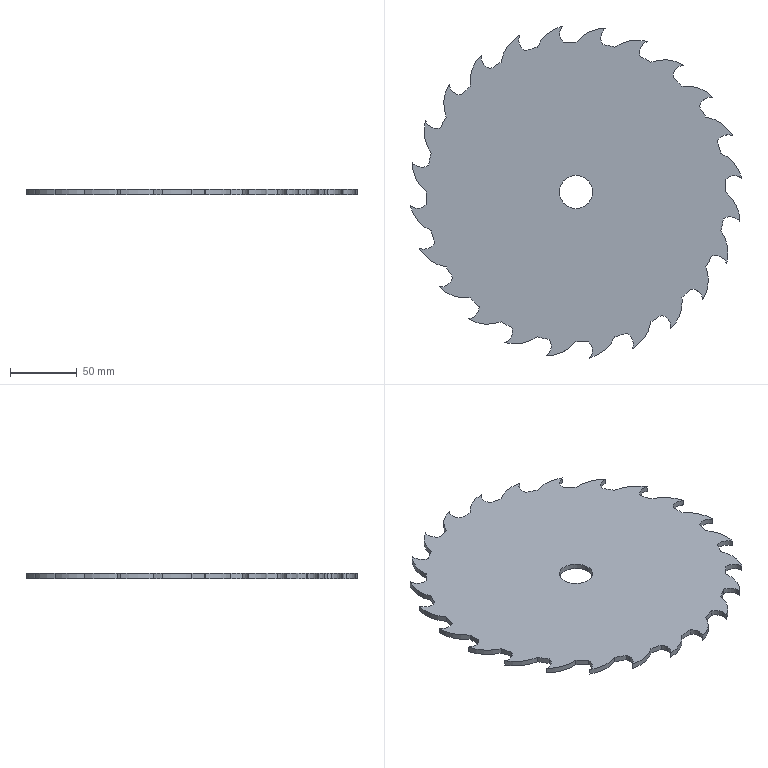Part | SolidWorks | features Extrusion 1 | 1 solid | 86 faces | box 249.174 x 249.174 x 4 mm | volume 170975 mm3 | cylinder 84 | plane 2 | commonest cylinder face diameters 17.678 x30 57.206 x28 225 x24 25 x2